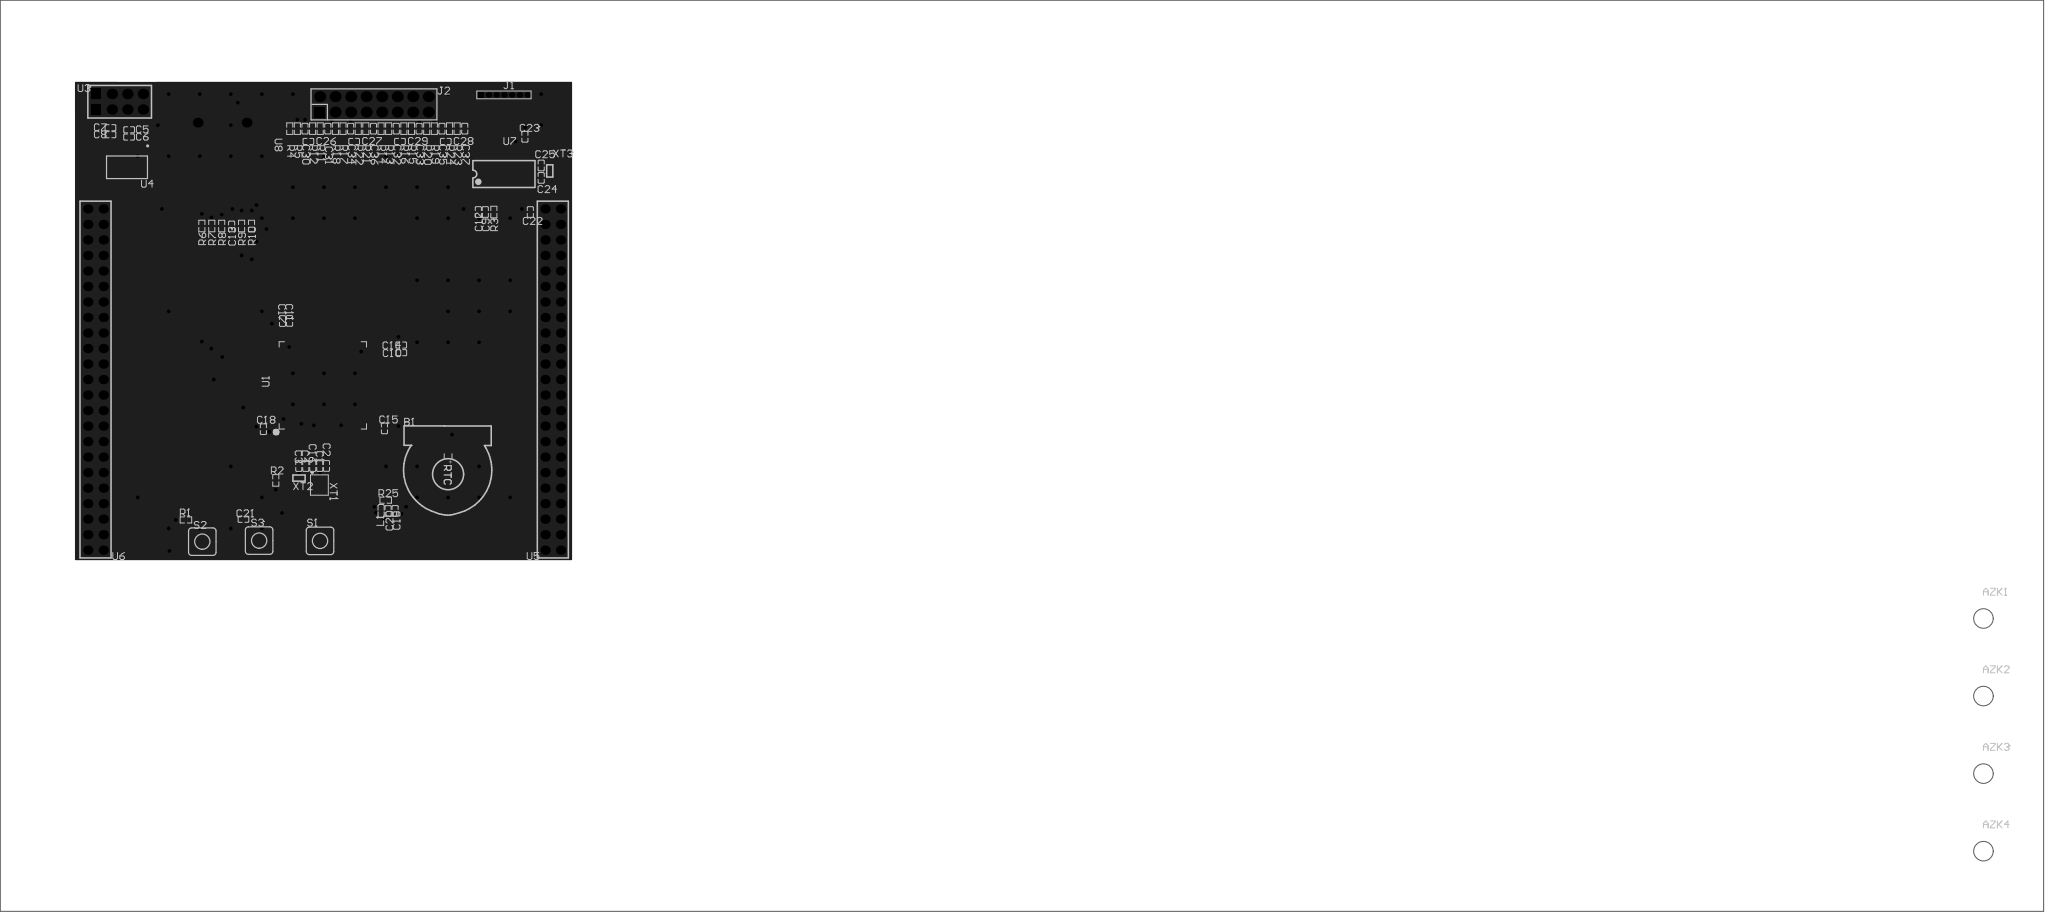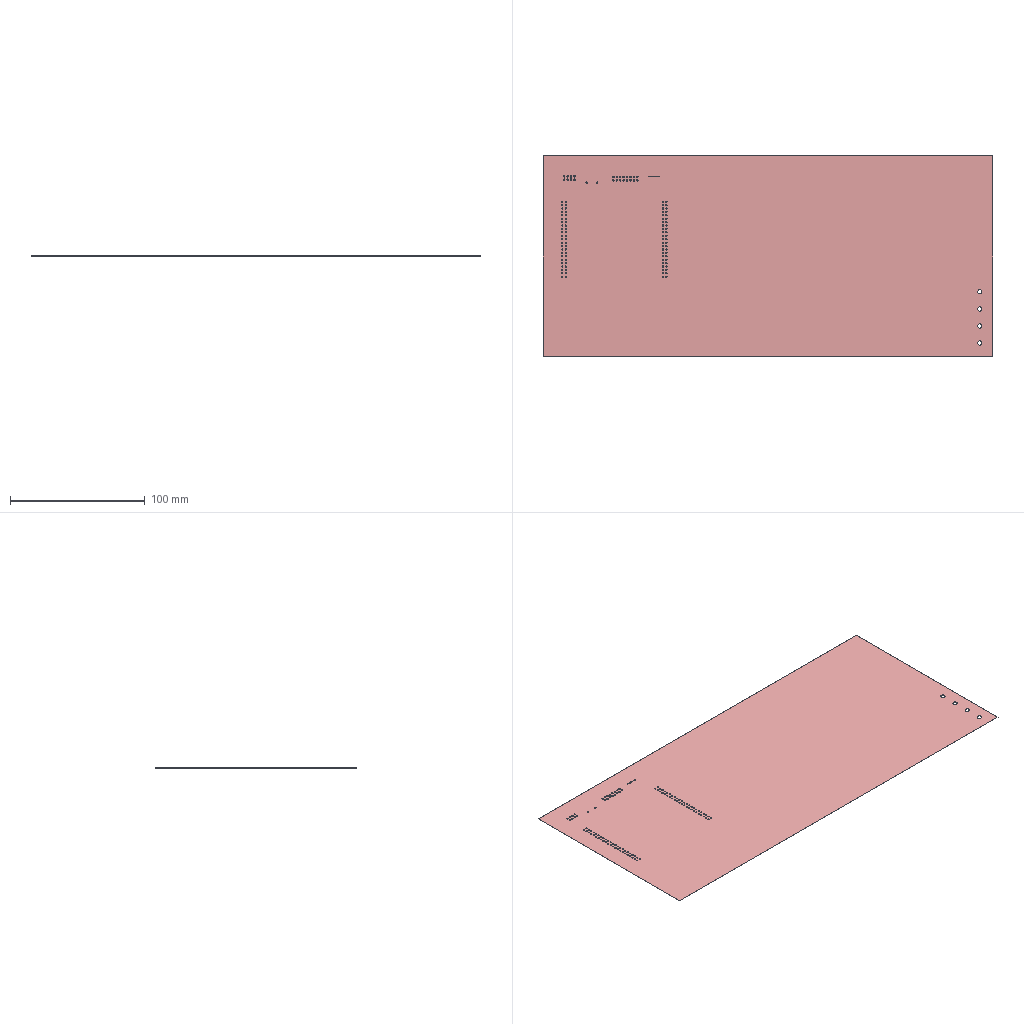Circuit board layout | Altium Designer | box 334.4 x 149.2 x 0.1 mm
Layer stack:
# Altium Designer layer stack of  (unit mm; dielectric type: 0 none, 1 core, 2 prepreg, 3 surface material)
index,name,kind,layer,copper_thickness_mm,dielectric_type,dielectric_thickness_mm,dielectric_material,dielectric_constant
0,Top Paste Mask Layer,other,,,,,,
1,Top Silkscreen Layer,other,,,,,,
2,Top Solder Mask Layer,dielectric,,,3,0.01,,3.3
3,Top Layer,copper,Top Layer,0.035,,,,
4,Bottom Layer,copper,Bottom Layer,0.035,,,,
5,Bottom Solder Mask Layer,dielectric,,,3,0.01,,3.3
6,Bottom Silkscreen Layer,other,,,,,,
7,Bottom Paste Mask Layer,other,,,,,,
# drill layer pairs: low layer,high layer
drill_pair,Top Layer,Bottom Layer
Part placement:
Designator,Comment,Layer,Footprint,Center-X(mm),Center-Y(mm),Rotation
AZK1,M3 mounting hole,TopLayer,M3安装孔(非金属化),0,0,0
AZK2,M3 mounting hole,TopLayer,M3安装孔(非金属化),0,0,0
AZK3,M3 mounting hole,TopLayer,M3安装孔(非金属化),0,0,0
AZK4,M3 mounting hole,TopLayer,M3安装孔(非金属化),0,0,0
B1,RTC,TopLayer,焊盘引出RTC,143.133,145.744,270
C1,22pF,TopLayer,C0402,122.127,142.763,90
C2,22pF,TopLayer,C0402,123.23,142.779,270
C3,3pF,TopLayer,C0402,118.698,142.763,270
C4,3pF,TopLayer,C0402,119.841,142.763,270
C5,10uF,TopLayer,C0402,90.932,197.82,180
C6,10uF,TopLayer,C0402,90.925,196.636,180
C7,10uF,TopLayer,C0402,87.877,198.16,180
C8,100nF,TopLayer,C0402,87.877,197.017,180
C9,47uF,TopLayer,C0402,149.225,184.358,90
C10,100pF,TopLayer,C0402,135.475,161.325,180
C11,100pF,TopLayer,C0402,117.187,166.532,270
C12,100nF,TopLayer,C0402,148.082,184.358,90
C13,100pF,TopLayer,C0402,107.709,181.997,90
C14,100pF,TopLayer,C0402,135.462,162.575,180
C15,100pF,TopLayer,C0402,132.715,148.925,90
C16,100pF,TopLayer,C0402,120.984,142.763,90
C17,100pF,TopLayer,C0402,116.031,166.512,270
C18,100pF,TopLayer,C0402,112.903,148.798,90
C19,100pF,TopLayer,C0402,134.459,135.417,90
C20,10uF,TopLayer,C0402,133.316,135.404,90
C21,100nF,TopLayer,C0402,109.645,134.05,180
C22,47uF,TopLayer,C0402,156.591,184.358,90
C23,100nF,TopLayer,C0402,155.702,196.677,270
C24,47uF,TopLayer,C0402,158.369,189.946,270
C25,47uF,TopLayer,C0402,158.369,191.978,90
C26,10nF,TopLayer,C0402,120.269,195.915,0
C27,10nF,TopLayer,C0402,127.762,195.915,0
C28,10nF,TopLayer,C0402,142.748,195.915,0
C29,10nF,TopLayer,C0402,135.255,195.915,0
C30,1nF,TopLayer,C0402,119.711,198.01,90
C31,1nF,TopLayer,C0402,123.447,198.01,90
C32,1nF,TopLayer,C0402,134.653,198.01,90
C33,1nF,TopLayer,C0402,138.389,198.01,90
C34,1nF,TopLayer,C0402,127.182,198.01,90
C35,1nF,TopLayer,C0402,142.125,198.01,90
C36,1nF,TopLayer,C0402,130.918,198.01,90
C37,1nF,TopLayer,C0402,145.86,198.01,90
J1,1.27 pin header 7p,TopLayer,1.27排针7P,152.273,203.535,0
J2,2.54 2*8P,TopLayer,HDR-TH_16P-P2.54-V-R2-C8-S2.54,131.003,201.984,0
L1,ferrite bead 600R,TopLayer,L0402,132.16,135.397,90
R1,10K,TopLayer,贴片电阻0402封装,100.226,133.939,0
R2,200R,TopLayer,贴片电阻0402封装,114.935,140.416,90
R3,0Ω,TopLayer,贴片电阻0402封装,150.622,184.358,90
R4,100Ω,TopLayer,贴片电阻0402封装,117.221,198.01,270
R5,10kΩ,TopLayer,贴片电阻0402封装,118.466,198.01,270
R6,10K,TopLayer,贴片电阻0402封装,102.833,182.067,90
R7,10K,TopLayer,贴片电阻0402封装,104.458,182.067,90
R8,10K,TopLayer,贴片电阻0402封装,106.083,182.067,90
R9,10K,TopLayer,贴片电阻0402封装,109.335,182.067,90
R10,10K,TopLayer,贴片电阻0402封装,110.961,182.067,90
R11,10kΩ,TopLayer,贴片电阻0402封装,122.201,198.01,270
R12,100Ω,TopLayer,贴片电阻0402封装,120.957,198.01,270
R13,10kΩ,TopLayer,贴片电阻0402封装,133.408,198.01,270
R14,100Ω,TopLayer,贴片电阻0402封装,132.163,198.01,270
R15,10kΩ,TopLayer,贴片电阻0402封装,137.143,198.01,270
R16,100Ω,TopLayer,贴片电阻0402封装,135.899,198.01,270
R17,10kΩ,TopLayer,贴片电阻0402封装,125.937,198.01,270
R18,100Ω,TopLayer,贴片电阻0402封装,124.692,198.01,270
R19,10kΩ,TopLayer,贴片电阻0402封装,140.879,198.01,270
R20,100Ω,TopLayer,贴片电阻0402封装,139.634,198.01,270
R21,10kΩ,TopLayer,贴片电阻0402封装,129.672,198.01,270
R22,100Ω,TopLayer,贴片电阻0402封装,128.428,198.01,270
R23,10kΩ,TopLayer,贴片电阻0402封装,144.614,198.01,270
R24,100Ω,TopLayer,贴片电阻0402封装,143.37,198.01,270
R25,0Ω,TopLayer,贴片电阻0402封装,132.922,137.175,180
S1,K_USER,TopLayer,按键开关4.5,122.174,130.51,270
S2,K_USER,TopLayer,按键开关4.5,102.906,130.383,270
S3,K_USER,TopLayer,按键开关4.5,112.209,130.555,270
U1,STM32H743VIT6,TopLayer,STM32H743VIT6,122.635,155.971,90
U3,HDR_2*4P,TopLayer,HDR_2*4P,89.383,202.417,90
U4,ASM1117,TopLayer,AMS1117-SOT-223,90.584,191.683,180
U7,ADS1256,TopLayer,SSOP-28_L10.2-W5.3-P0.65-LS7.8-BL,152.272,190.578,0
U8,MICRO SD TF card socket,TopLayer,MICRO_SD_TF¿¨×ù,105.311,193.446,270
XT1,XTAL3225,TopLayer,XTAL3225,122.047,139.654,270
XT2,32.768k,TopLayer,SMD-2012_2P,118.745,140.797,0
XT3,7.68MHz,TopLayer,SMD-2012_2P,159.766,191.089,90
U5,STM32H7,TopLayer,2*23,160.274,156.926,180
U6,STM32H7,TopLayer,2*23,85.434,156.926,180
Pad and via stacks:
# Altium Designer via and pad stacks of  (unit mm). Each distinct definition once, with the count of objects using it.
# via: kind,start_layer,end_layer,hole_mm,diameter_mm,mode(0 simple;1 top-mid-bottom;2 full stack),diameter_per_layer,count,example_net
# pad: kind,layer,hole_mm,hole_type(0 round;1 square;2 slot),plating,top_size,top_shape(1 round;2 rect;3 octagon;9 rounded rect),mid_size,bottom_size,mode,footprint,size_per_layer,count,example
pad,Top Layer,0,0,plated,1.524x0.508,2,1.524x0.508,1.524x0.508,0,\u00BA\u00B8\u00C5\u00CC\u00D2\u00FD\u00B3\u00F6RTC,,2,B1.1
pad,Top Layer,0,0,plated,0.5x0.54,2,0.5x0.54,0.5x0.54,0,C0402,,74,C1.2
pad,Top Layer,0,0,plated,0.54x0.54,2,0.54x0.54,0.54x0.54,0,L0402,,2,L1.2
pad,Top Layer,0,0,plated,0.5657x0.54,2,0.5657x0.54,0.5657x0.54,0,\u00CC\u00F9\u00C6\u00AC\u00B5\u00E7\u00D7\u00E80402\u00B7\u00E2\u00D7\u00B0,,50,R1.2
pad,Top Layer,0,0,plated,0.5x0.5,1,0.5x0.5,0.5x0.5,0,\u00B0\u00B4\u00BC\u00FC\u00BF\u00AA\u00B9\u00D84.5,,12,S1.4
pad,Top Layer,0,0,plated,0.27x1.2,1,0.27x1.2,0.27x1.2,0,STM32H743VIT6,,100,U1.1
pad,Top Layer,0,0,plated,3.5x1.75,2,3.5x1.75,3.5x1.75,0,AMS1117-SOT-223,,1,U4.4
pad,Top Layer,0,0,plated,1.1x1.75,2,1.1x1.75,1.1x1.75,0,AMS1117-SOT-223,,3,U4.3
pad,Top Layer,0,0,plated,0.364x2.015,1,0.364x2.015,0.364x2.015,0,SSOP-28_L10.2-W5.3-P0.65-LS7.8-BL,,28,U7.1
pad,Top Layer,0,0,plated,2x0.5,2,2x0.5,2x0.5,0,MICRO SD TF\u00BF\u00A8\u00D7\u00F9,,9,U8.1
pad,Top Layer,0,0,plated,1.6x1.8,2,1.6x1.8,1.6x1.8,0,MICRO SD TF\u00BF\u00A8\u00D7\u00F9,,1,U8.6
pad,Top Layer,0,0,plated,2.4x1.6,2,2.4x1.6,2.4x1.6,0,MICRO SD TF\u00BF\u00A8\u00D7\u00F9,,2,U8.6
pad,Top Layer,0,0,plated,1.399x1.801,2,1.399x1.801,1.399x1.801,0,MICRO SD TF\u00BF\u00A8\u00D7\u00F9,,1,U8.6
pad,Top Layer,0,0,plated,1.1x1,2,1.1x1,1.1x1,0,XTAL3225,,4,XT1.4
pad,Top Layer,0,0,plated,1.2x0.8,2,1.2x0.8,1.2x0.8,0,SMD-2012_2P,,4,XT2.1
pad,Multi-Layer,0.6,0,plated,0.9x0.9,2,0.9x0.9,0.9x0.9,0,1.27\u00C5\u00C5\u00D5\u00EB7P,,1,J1.1
pad,Multi-Layer,0.6,0,plated,0.9x0.9,1,0.9x0.9,0.9x0.9,0,1.27\u00C5\u00C5\u00D5\u00EB7P,,6,J1.2
pad,Multi-Layer,1.1,0,plated,1.8x1.8,1,1.8x1.8,1.8x1.8,0,HDR-TH_16P-P2.54-V-R2-C8-S2.54,,15,J2.16
pad,Multi-Layer,1.1,0,plated,1.8x1.8,2,1.8x1.8,1.8x1.8,0,HDR-TH_16P-P2.54-V-R2-C8-S2.54,,1,J2.1
pad,Multi-Layer,1.1,0,plated,1.7x1.7,1,1.7x1.7,1.7x1.7,0,HDR_2*4P,,6,U3.3
pad,Multi-Layer,1.1,0,plated,1.7x1.524,2,1.7x1.524,1.7x1.524,0,HDR_2*4P,,2,U3.1
pad,Multi-Layer,1,0,plated,1.6x1.6,1,1.6x1.6,1.6x1.6,0,MICRO SD TF\u00BF\u00A8\u00D7\u00F9,,2,U8.6
pad,Multi-Layer,0.9144,0,plated,1.524x1.524,1,1.524x1.524,1.524x1.524,0,2*23,,92,U5.1
via,Top Layer,Bottom Layer,0.3048,0.61,0,,55,BOOT0
via,Top Layer,Bottom Layer,0.3048,0.6096,0,,65,GND
Copper pours:
name,layer,net,type(0 solid;1 hatched;2 none)
Bottom Layer-GND,Bottom Layer,GND,0
Top Layer-GND,Top Layer,GND,0
Design rules, without the lines most boards share:
# Altium Designer design rules of  (exported by Altium Designer, unit mm)
# columns: name | kind | enabled | priority | scope1 | scope2 | descriptor | typed fields (field=value)
Default | 0 | enabled | 1 | All | All | Clearance Constraint (Gap=6mil) (All),(All) | gap=0.1524
Default_1 | 63 | enabled | 1 | All | All | Board Clearance Constraint (Gap=0mil) (All) |
otherClearance | 52 | enabled | 1 | All | All | Hole To Hole Clearance (Gap=11.8mil) (All),(All) | gap=0.2997
Default_2 | 2 | enabled | 1 | All | All | Width Constraint (Min=10mil) (Max=1000mil) (Preferred=10mil) (All) |
differentialPair | 51 | enabled | 1 | All | All | Differential Pairs Uncoupled Length using the Gap Constraints (Min=5mil) (Max=6mil) (Prefered=6mil)  and Width Constraints (Min=5mil) (Max=100mil) (Prefered=100mil) (All) |
Default_3 | 11 | enabled | 1 | All | All | Routing Via (MinHoleWidth=12mil) (MaxHoleWidth=1181mil) (PreferredHoleWidth=12mil) (MinWidth=24mil) (MaxWidth=1969mil) (PreferedWidth=24mil) (All) | via_min_hole=0.3048 via_max_hole=29.997 via_preferred_diameter=0.6096 via_preferred_hole=0.3048
Common | 13 | enabled | 2 | All | All | Solder Mask Expansion (Expansion =2mil) (All) | expansion=0.0508
Common_1 | 13 | enabled | 1 | IsVia | All | Solder Mask Expansion (Expansion =-1000mil) (IsVia) | expansion=-25.4